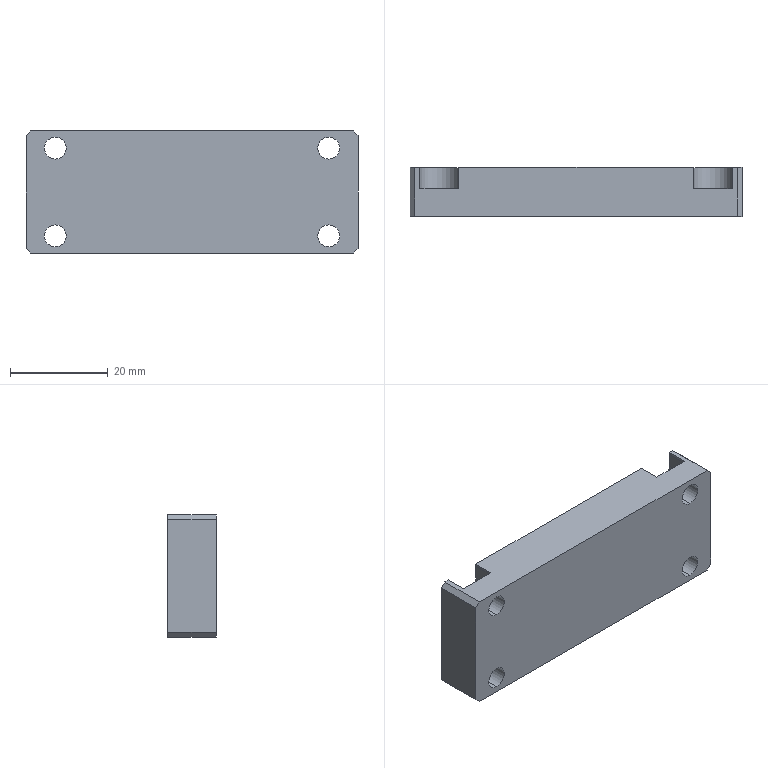Part | SolidWorks | features Chamfer 1, Extrusion 1, HoleWzd 1, ICE 1 | 1 solid | 44 faces | box 68 x 10 x 25 mm | volume 15689 mm3 | cylinder 22 | plane 22 | commonest cylinder face diameters 8 x14 4.5 x8
STEP:
#1=CARTESIAN_POINT('',(-28.,-5.,-11.25));
#2=VERTEX_POINT('',#1);
#3=CARTESIAN_POINT('',(-28.,-5.,-6.75));
#4=VERTEX_POINT('',#3);
#5=CARTESIAN_POINT('',(-28.,-5.,-9.));
#6=DIRECTION('',(0.,1.,0.));
#7=DIRECTION('',(0.,0.,1.));
#8=AXIS2_PLACEMENT_3D('',#5,#6,#7);
#9=CIRCLE('',#8,2.25);
#10=EDGE_CURVE('',#2,#4,#9,.T.);
#11=ORIENTED_EDGE('',*,*,#10,.F.);
#12=CARTESIAN_POINT('',(-28.,0.6,-11.25));
#13=VERTEX_POINT('',#12);
#14=CARTESIAN_POINT('',(-28.,5.,-11.25));
#15=DIRECTION('',(0.,1.,0.));
#16=VECTOR('',#15,1000.);
#17=LINE('',#14,#16);
#18=EDGE_CURVE('',#2,#13,#17,.T.);
#19=ORIENTED_EDGE('',*,*,#18,.T.);
#20=CARTESIAN_POINT('',(-28.,0.6,-6.75));
#21=VERTEX_POINT('',#20);
#22=CARTESIAN_POINT('',(-28.,0.6,-9.));
#23=DIRECTION('',(0.,1.,0.));
#24=DIRECTION('',(0.,0.,1.));
#25=AXIS2_PLACEMENT_3D('',#22,#23,#24);
#26=CIRCLE('',#25,2.25);
#27=EDGE_CURVE('',#13,#21,#26,.T.);
#28=ORIENTED_EDGE('',*,*,#27,.T.);
#29=CARTESIAN_POINT('',(-28.,5.,-6.75));
#30=DIRECTION('',(0.,1.,0.));
#31=VECTOR('',#30,1000.);
#32=LINE('',#29,#31);
#33=EDGE_CURVE('',#4,#21,#32,.T.);
#34=ORIENTED_EDGE('',*,*,#33,.F.);
#35=EDGE_LOOP('',(#11,#19,#28,#34));
#36=FACE_OUTER_BOUND('',#35,.T.);
#37=CARTESIAN_POINT('',(-28.,5.,-9.));
#38=DIRECTION('',(0.,1.,0.));
#39=DIRECTION('',(0.,0.,1.));
#40=AXIS2_PLACEMENT_3D('',#37,#38,#39);
#41=CYLINDRICAL_SURFACE('',#40,2.25);
#42=ADVANCED_FACE('',(#36),#41,.F.);
#43=CARTESIAN_POINT('',(-28.,-5.,6.75));
#44=VERTEX_POINT('',#43);
#45=CARTESIAN_POINT('',(-28.,-5.,11.25));
#46=VERTEX_POINT('',#45);
#47=CARTESIAN_POINT('',(-28.,-5.,9.));
#48=DIRECTION('',(0.,1.,0.));
#49=DIRECTION('',(0.,0.,1.));
#50=AXIS2_PLACEMENT_3D('',#47,#48,#49);
#51=CIRCLE('',#50,2.25);
#52=EDGE_CURVE('',#44,#46,#51,.T.);
#53=ORIENTED_EDGE('',*,*,#52,.F.);
#54=CARTESIAN_POINT('',(-28.,0.6,6.75));
#55=VERTEX_POINT('',#54);
#56=CARTESIAN_POINT('',(-28.,5.,6.75));
#57=DIRECTION('',(0.,1.,0.));
#58=VECTOR('',#57,1000.);
#59=LINE('',#56,#58);
#60=EDGE_CURVE('',#44,#55,#59,.T.);
#61=ORIENTED_EDGE('',*,*,#60,.T.);
#62=CARTESIAN_POINT('',(-28.,0.6,11.25));
#63=VERTEX_POINT('',#62);
#64=CARTESIAN_POINT('',(-28.,0.6,9.));
#65=DIRECTION('',(0.,1.,0.));
#66=DIRECTION('',(0.,0.,1.));
#67=AXIS2_PLACEMENT_3D('',#64,#65,#66);
#68=CIRCLE('',#67,2.25);
#69=EDGE_CURVE('',#55,#63,#68,.T.);
#70=ORIENTED_EDGE('',*,*,#69,.T.);
#71=CARTESIAN_POINT('',(-28.,5.,11.25));
#72=DIRECTION('',(0.,1.,0.));
#73=VECTOR('',#72,1000.);
#74=LINE('',#71,#73);
#75=EDGE_CURVE('',#46,#63,#74,.T.);
#76=ORIENTED_EDGE('',*,*,#75,.F.);
#77=EDGE_LOOP('',(#53,#61,#70,#76));
#78=FACE_OUTER_BOUND('',#77,.T.);
#79=CARTESIAN_POINT('',(-28.,5.,9.));
#80=DIRECTION('',(0.,1.,0.));
#81=DIRECTION('',(0.,0.,1.));
#82=AXIS2_PLACEMENT_3D('',#79,#80,#81);
#83=CYLINDRICAL_SURFACE('',#82,2.25);
#84=ADVANCED_FACE('',(#78),#83,.F.);
#85=CARTESIAN_POINT('',(28.,-5.,-11.25));
#86=VERTEX_POINT('',#85);
#87=CARTESIAN_POINT('',(28.,-5.,-6.75));
#88=VERTEX_POINT('',#87);
#89=CARTESIAN_POINT('',(28.,-5.,-9.));
#90=DIRECTION('',(0.,1.,0.));
#91=DIRECTION('',(0.,0.,1.));
#92=AXIS2_PLACEMENT_3D('',#89,#90,#91);
#93=CIRCLE('',#92,2.25);
#94=EDGE_CURVE('',#86,#88,#93,.T.);
#95=ORIENTED_EDGE('',*,*,#94,.F.);
#96=CARTESIAN_POINT('',(28.,0.6,-11.25));
#97=VERTEX_POINT('',#96);
#98=CARTESIAN_POINT('',(28.,5.,-11.25));
#99=DIRECTION('',(0.,1.,0.));
#100=VECTOR('',#99,1000.);
#101=LINE('',#98,#100);
#102=EDGE_CURVE('',#86,#97,#101,.T.);
#103=ORIENTED_EDGE('',*,*,#102,.T.);
#104=CARTESIAN_POINT('',(28.,0.6,-6.75));
#105=VERTEX_POINT('',#104);
#106=CARTESIAN_POINT('',(28.,0.6,-9.));
#107=DIRECTION('',(0.,1.,0.));
#108=DIRECTION('',(0.,0.,1.));
#109=AXIS2_PLACEMENT_3D('',#106,#107,#108);
#110=CIRCLE('',#109,2.25);
#111=EDGE_CURVE('',#97,#105,#110,.T.);
#112=ORIENTED_EDGE('',*,*,#111,.T.);
#113=CARTESIAN_POINT('',(28.,5.,-6.75));
#114=DIRECTION('',(0.,1.,0.));
#115=VECTOR('',#114,1000.);
#116=LINE('',#113,#115);
#117=EDGE_CURVE('',#88,#105,#116,.T.);
#118=ORIENTED_EDGE('',*,*,#117,.F.);
#119=EDGE_LOOP('',(#95,#103,#112,#118));
#120=FACE_OUTER_BOUND('',#119,.T.);
#121=CARTESIAN_POINT('',(28.,5.,-9.));
#122=DIRECTION('',(0.,1.,0.));
#123=DIRECTION('',(0.,0.,1.));
#124=AXIS2_PLACEMENT_3D('',#121,#122,#123);
#125=CYLINDRICAL_SURFACE('',#124,2.25);
#126=ADVANCED_FACE('',(#120),#125,.F.);
#127=CARTESIAN_POINT('',(28.,-5.,6.75));
#128=VERTEX_POINT('',#127);
#129=CARTESIAN_POINT('',(28.,-5.,11.25));
#130=VERTEX_POINT('',#129);
#131=CARTESIAN_POINT('',(28.,-5.,9.));
#132=DIRECTION('',(0.,1.,0.));
#133=DIRECTION('',(0.,0.,1.));
#134=AXIS2_PLACEMENT_3D('',#131,#132,#133);
#135=CIRCLE('',#134,2.25);
#136=EDGE_CURVE('',#128,#130,#135,.T.);
#137=ORIENTED_EDGE('',*,*,#136,.F.);
#138=CARTESIAN_POINT('',(28.,0.6,6.75));
#139=VERTEX_POINT('',#138);
#140=CARTESIAN_POINT('',(28.,5.,6.75));
#141=DIRECTION('',(0.,1.,0.));
#142=VECTOR('',#141,1000.);
#143=LINE('',#140,#142);
#144=EDGE_CURVE('',#128,#139,#143,.T.);
#145=ORIENTED_EDGE('',*,*,#144,.T.);
#146=CARTESIAN_POINT('',(28.,0.6,11.25));
#147=VERTEX_POINT('',#146);
#148=CARTESIAN_POINT('',(28.,0.6,9.));
#149=DIRECTION('',(0.,1.,0.));
#150=DIRECTION('',(0.,0.,1.));
#151=AXIS2_PLACEMENT_3D('',#148,#149,#150);
#152=CIRCLE('',#151,2.25);
#153=EDGE_CURVE('',#139,#147,#152,.T.);
#154=ORIENTED_EDGE('',*,*,#153,.T.);
#155=CARTESIAN_POINT('',(28.,5.,11.25));
#156=DIRECTION('',(0.,1.,0.));
#157=VECTOR('',#156,1000.);
#158=LINE('',#155,#157);
#159=EDGE_CURVE('',#130,#147,#158,.T.);
#160=ORIENTED_EDGE('',*,*,#159,.F.);
#161=EDGE_LOOP('',(#137,#145,#154,#160));
#162=FACE_OUTER_BOUND('',#161,.T.);
#163=CARTESIAN_POINT('',(28.,5.,9.));
#164=DIRECTION('',(0.,1.,0.));
#165=DIRECTION('',(0.,0.,1.));
#166=AXIS2_PLACEMENT_3D('',#163,#164,#165);
#167=CYLINDRICAL_SURFACE('',#166,2.25);
#168=ADVANCED_FACE('',(#162),#167,.F.);
#169=CARTESIAN_POINT('',(-28.,0.6,-5.));
#170=VERTEX_POINT('',#169);
#171=CARTESIAN_POINT('',(-24.,0.6,-9.));
#172=VERTEX_POINT('',#171);
#173=CARTESIAN_POINT('',(-28.,0.6,-9.));
#174=DIRECTION('',(0.,1.,0.));
#175=DIRECTION('',(0.,0.,1.));
#176=AXIS2_PLACEMENT_3D('',#173,#174,#175);
#177=CIRCLE('',#176,4.);
#178=EDGE_CURVE('',#170,#172,#177,.T.);
#179=ORIENTED_EDGE('',*,*,#178,.F.);
#180=CARTESIAN_POINT('',(-28.,5.,-5.));
#181=VERTEX_POINT('',#180);
#182=CARTESIAN_POINT('',(-28.,5.,-5.));
#183=DIRECTION('',(0.,1.,0.));
#184=VECTOR('',#183,1000.);
#185=LINE('',#182,#184);
#186=EDGE_CURVE('',#170,#181,#185,.T.);
#187=ORIENTED_EDGE('',*,*,#186,.T.);
#188=CARTESIAN_POINT('',(-24.,5.,-9.));
#189=VERTEX_POINT('',#188);
#190=CARTESIAN_POINT('',(-28.,5.,-9.));
#191=DIRECTION('',(0.,1.,0.));
#192=DIRECTION('',(0.,0.,1.));
#193=AXIS2_PLACEMENT_3D('',#190,#191,#192);
#194=CIRCLE('',#193,4.);
#195=EDGE_CURVE('',#181,#189,#194,.T.);
#196=ORIENTED_EDGE('',*,*,#195,.T.);
#197=CARTESIAN_POINT('',(-24.,-13.001,-9.));
#198=DIRECTION('',(0.,1.,0.));
#199=VECTOR('',#198,1000.);
#200=LINE('',#197,#199);
#201=EDGE_CURVE('',#172,#189,#200,.T.);
#202=ORIENTED_EDGE('',*,*,#201,.F.);
#203=EDGE_LOOP('',(#179,#187,#196,#202));
#204=FACE_OUTER_BOUND('',#203,.T.);
#205=CARTESIAN_POINT('',(-28.,5.,-9.));
#206=DIRECTION('',(0.,1.,0.));
#207=DIRECTION('',(0.,0.,1.));
#208=AXIS2_PLACEMENT_3D('',#205,#206,#207);
#209=CYLINDRICAL_SURFACE('',#208,4.);
#210=ADVANCED_FACE('',(#204),#209,.F.);
#211=CARTESIAN_POINT('',(28.,0.6,-5.));
#212=VERTEX_POINT('',#211);
#213=CARTESIAN_POINT('',(32.,0.6,-9.));
#214=VERTEX_POINT('',#213);
#215=CARTESIAN_POINT('',(28.,0.6,-9.));
#216=DIRECTION('',(0.,1.,0.));
#217=DIRECTION('',(0.,0.,1.));
#218=AXIS2_PLACEMENT_3D('',#215,#216,#217);
#219=CIRCLE('',#218,4.);
#220=EDGE_CURVE('',#212,#214,#219,.T.);
#221=ORIENTED_EDGE('',*,*,#220,.F.);
#222=CARTESIAN_POINT('',(28.,5.,-5.));
#223=VERTEX_POINT('',#222);
#224=CARTESIAN_POINT('',(28.,5.,-5.));
#225=DIRECTION('',(0.,1.,0.));
#226=VECTOR('',#225,1000.);
#227=LINE('',#224,#226);
#228=EDGE_CURVE('',#212,#223,#227,.T.);
#229=ORIENTED_EDGE('',*,*,#228,.T.);
#230=CARTESIAN_POINT('',(32.,5.,-9.));
#231=VERTEX_POINT('',#230);
#232=CARTESIAN_POINT('',(28.,5.,-9.));
#233=DIRECTION('',(0.,1.,0.));
#234=DIRECTION('',(0.,0.,1.));
#235=AXIS2_PLACEMENT_3D('',#232,#233,#234);
#236=CIRCLE('',#235,4.);
#237=EDGE_CURVE('',#223,#231,#236,.T.);
#238=ORIENTED_EDGE('',*,*,#237,.T.);
#239=CARTESIAN_POINT('',(32.,-13.001,-9.));
#240=DIRECTION('',(0.,1.,0.));
#241=VECTOR('',#240,1000.);
#242=LINE('',#239,#241);
#243=EDGE_CURVE('',#214,#231,#242,.T.);
#244=ORIENTED_EDGE('',*,*,#243,.F.);
#245=EDGE_LOOP('',(#221,#229,#238,#244));
#246=FACE_OUTER_BOUND('',#245,.T.);
#247=CARTESIAN_POINT('',(28.,5.,-9.));
#248=DIRECTION('',(0.,1.,0.));
#249=DIRECTION('',(0.,0.,1.));
#250=AXIS2_PLACEMENT_3D('',#247,#248,#249);
#251=CYLINDRICAL_SURFACE('',#250,4.);
#252=ADVANCED_FACE('',(#246),#251,.F.);
#253=CARTESIAN_POINT('',(32.,5.,9.));
#254=VERTEX_POINT('',#253);
#255=CARTESIAN_POINT('',(24.,5.,9.));
#256=VERTEX_POINT('',#255);
#257=CARTESIAN_POINT('',(28.,5.,9.));
#258=DIRECTION('',(0.,1.,0.));
#259=DIRECTION('',(0.,0.,1.));
#260=AXIS2_PLACEMENT_3D('',#257,#258,#259);
#261=CIRCLE('',#260,4.);
#262=EDGE_CURVE('',#254,#256,#261,.T.);
#263=ORIENTED_EDGE('',*,*,#262,.T.);
#264=CARTESIAN_POINT('',(24.,0.6,9.));
#265=VERTEX_POINT('',#264);
#266=CARTESIAN_POINT('',(24.,-13.001,9.));
#267=DIRECTION('',(0.,1.,0.));
#268=VECTOR('',#267,1000.);
#269=LINE('',#266,#268);
#270=EDGE_CURVE('',#265,#256,#269,.T.);
#271=ORIENTED_EDGE('',*,*,#270,.F.);
#272=CARTESIAN_POINT('',(32.,0.6,9.));
#273=VERTEX_POINT('',#272);
#274=CARTESIAN_POINT('',(28.,0.6,9.));
#275=DIRECTION('',(0.,1.,0.));
#276=DIRECTION('',(0.,0.,1.));
#277=AXIS2_PLACEMENT_3D('',#274,#275,#276);
#278=CIRCLE('',#277,4.);
#279=EDGE_CURVE('',#273,#265,#278,.T.);
#280=ORIENTED_EDGE('',*,*,#279,.F.);
#281=CARTESIAN_POINT('',(32.,-13.001,9.));
#282=DIRECTION('',(0.,1.,0.));
#283=VECTOR('',#282,1000.);
#284=LINE('',#281,#283);
#285=EDGE_CURVE('',#273,#254,#284,.T.);
#286=ORIENTED_EDGE('',*,*,#285,.T.);
#287=EDGE_LOOP('',(#263,#271,#280,#286));
#288=FACE_OUTER_BOUND('',#287,.T.);
#289=CARTESIAN_POINT('',(28.,5.,9.));
#290=DIRECTION('',(0.,1.,0.));
#291=DIRECTION('',(0.,0.,1.));
#292=AXIS2_PLACEMENT_3D('',#289,#290,#291);
#293=CYLINDRICAL_SURFACE('',#292,4.);
#294=ADVANCED_FACE('',(#288),#293,.F.);
#295=ORIENTED_EDGE('',*,*,#228,.F.);
#296=CARTESIAN_POINT('',(24.,0.6,-9.));
#297=VERTEX_POINT('',#296);
#298=CARTESIAN_POINT('',(28.,0.6,-9.));
#299=DIRECTION('',(0.,1.,0.));
#300=DIRECTION('',(0.,0.,1.));
#301=AXIS2_PLACEMENT_3D('',#298,#299,#300);
#302=CIRCLE('',#301,4.);
#303=EDGE_CURVE('',#297,#212,#302,.T.);
#304=ORIENTED_EDGE('',*,*,#303,.F.);
#305=CARTESIAN_POINT('',(24.,5.,-9.));
#306=VERTEX_POINT('',#305);
#307=CARTESIAN_POINT('',(24.,-13.001,-9.));
#308=DIRECTION('',(0.,1.,0.));
#309=VECTOR('',#308,1000.);
#310=LINE('',#307,#309);
#311=EDGE_CURVE('',#297,#306,#310,.T.);
#312=ORIENTED_EDGE('',*,*,#311,.T.);
#313=CARTESIAN_POINT('',(28.,5.,-9.));
#314=DIRECTION('',(0.,1.,0.));
#315=DIRECTION('',(0.,0.,1.));
#316=AXIS2_PLACEMENT_3D('',#313,#314,#315);
#317=CIRCLE('',#316,4.);
#318=EDGE_CURVE('',#306,#223,#317,.T.);
#319=ORIENTED_EDGE('',*,*,#318,.T.);
#320=EDGE_LOOP('',(#295,#304,#312,#319));
#321=FACE_OUTER_BOUND('',#320,.T.);
#322=CARTESIAN_POINT('',(28.,5.,-9.));
#323=DIRECTION('',(0.,1.,0.));
#324=DIRECTION('',(0.,0.,1.));
#325=AXIS2_PLACEMENT_3D('',#322,#323,#324);
#326=CYLINDRICAL_SURFACE('',#325,4.);
#327=ADVANCED_FACE('',(#321),#326,.F.);
#328=CARTESIAN_POINT('',(-24.,5.,9.));
#329=VERTEX_POINT('',#328);
#330=CARTESIAN_POINT('',(-32.,5.,9.));
#331=VERTEX_POINT('',#330);
#332=CARTESIAN_POINT('',(-28.,5.,9.));
#333=DIRECTION('',(0.,1.,0.));
#334=DIRECTION('',(0.,0.,1.));
#335=AXIS2_PLACEMENT_3D('',#332,#333,#334);
#336=CIRCLE('',#335,4.);
#337=EDGE_CURVE('',#329,#331,#336,.T.);
#338=ORIENTED_EDGE('',*,*,#337,.T.);
#339=CARTESIAN_POINT('',(-32.,0.6,9.));
#340=VERTEX_POINT('',#339);
#341=CARTESIAN_POINT('',(-32.,-13.001,9.));
#342=DIRECTION('',(0.,1.,0.));
#343=VECTOR('',#342,1000.);
#344=LINE('',#341,#343);
#345=EDGE_CURVE('',#340,#331,#344,.T.);
#346=ORIENTED_EDGE('',*,*,#345,.F.);
#347=CARTESIAN_POINT('',(-24.,0.6,9.));
#348=VERTEX_POINT('',#347);
#349=CARTESIAN_POINT('',(-28.,0.6,9.));
#350=DIRECTION('',(0.,1.,0.));
#351=DIRECTION('',(0.,0.,1.));
#352=AXIS2_PLACEMENT_3D('',#349,#350,#351);
#353=CIRCLE('',#352,4.);
#354=EDGE_CURVE('',#348,#340,#353,.T.);
#355=ORIENTED_EDGE('',*,*,#354,.F.);
#356=CARTESIAN_POINT('',(-24.,-13.001,9.));
#357=DIRECTION('',(0.,1.,0.));
#358=VECTOR('',#357,1000.);
#359=LINE('',#356,#358);
#360=EDGE_CURVE('',#348,#329,#359,.T.);
#361=ORIENTED_EDGE('',*,*,#360,.T.);
#362=EDGE_LOOP('',(#338,#346,#355,#361));
#363=FACE_OUTER_BOUND('',#362,.T.);
#364=CARTESIAN_POINT('',(-28.,5.,9.));
#365=DIRECTION('',(0.,1.,0.));
#366=DIRECTION('',(0.,0.,1.));
#367=AXIS2_PLACEMENT_3D('',#364,#365,#366);
#368=CYLINDRICAL_SURFACE('',#367,4.);
#369=ADVANCED_FACE('',(#363),#368,.F.);
#370=ORIENTED_EDGE('',*,*,#186,.F.);
#371=CARTESIAN_POINT('',(-32.,0.6,-9.));
#372=VERTEX_POINT('',#371);
#373=CARTESIAN_POINT('',(-28.,0.6,-9.));
#374=DIRECTION('',(0.,1.,0.));
#375=DIRECTION('',(0.,0.,1.));
#376=AXIS2_PLACEMENT_3D('',#373,#374,#375);
#377=CIRCLE('',#376,4.);
#378=EDGE_CURVE('',#372,#170,#377,.T.);
#379=ORIENTED_EDGE('',*,*,#378,.F.);
#380=CARTESIAN_POINT('',(-32.,5.,-9.));
#381=VERTEX_POINT('',#380);
#382=CARTESIAN_POINT('',(-32.,-13.001,-9.));
#383=DIRECTION('',(0.,1.,0.));
#384=VECTOR('',#383,1000.);
#385=LINE('',#382,#384);
#386=EDGE_CURVE('',#372,#381,#385,.T.);
#387=ORIENTED_EDGE('',*,*,#386,.T.);
#388=CARTESIAN_POINT('',(-28.,5.,-9.));
#389=DIRECTION('',(0.,1.,0.));
#390=DIRECTION('',(0.,0.,1.));
#391=AXIS2_PLACEMENT_3D('',#388,#389,#390);
#392=CIRCLE('',#391,4.);
#393=EDGE_CURVE('',#381,#181,#392,.T.);
#394=ORIENTED_EDGE('',*,*,#393,.T.);
#395=EDGE_LOOP('',(#370,#379,#387,#394));
#396=FACE_OUTER_BOUND('',#395,.T.);
#397=CARTESIAN_POINT('',(-28.,5.,-9.));
#398=DIRECTION('',(0.,1.,0.));
#399=DIRECTION('',(0.,0.,1.));
#400=AXIS2_PLACEMENT_3D('',#397,#398,#399);
#401=CYLINDRICAL_SURFACE('',#400,4.);
#402=ADVANCED_FACE('',(#396),#401,.F.);
#403=CARTESIAN_POINT('',(34.,-5.,11.5));
#404=VERTEX_POINT('',#403);
#405=CARTESIAN_POINT('',(34.,-5.,-11.5));
#406=VERTEX_POINT('',#405);
#407=CARTESIAN_POINT('',(34.,-5.,-12.5));
#408=DIRECTION('',(0.,0.,-1.));
#409=VECTOR('',#408,1000.);
#410=LINE('',#407,#409);
#411=EDGE_CURVE('',#404,#406,#410,.T.);
#412=ORIENTED_EDGE('',*,*,#411,.T.);
#413=CARTESIAN_POINT('',(34.,5.,-11.5));
#414=VERTEX_POINT('',#413);
#415=CARTESIAN_POINT('',(34.,5.,-11.5));
#416=DIRECTION('',(0.,1.,0.));
#417=VECTOR('',#416,1000.);
#418=LINE('',#415,#417);
#419=EDGE_CURVE('',#406,#414,#418,.T.);
#420=ORIENTED_EDGE('',*,*,#419,.T.);
#421=CARTESIAN_POINT('',(34.,5.,11.5));
#422=VERTEX_POINT('',#421);
#423=CARTESIAN_POINT('',(34.,5.,-12.5));
#424=DIRECTION('',(0.,0.,-1.));
#425=VECTOR('',#424,1000.);
#426=LINE('',#423,#425);
#427=EDGE_CURVE('',#422,#414,#426,.T.);
#428=ORIENTED_EDGE('',*,*,#427,.F.);
#429=CARTESIAN_POINT('',(34.,5.,11.5));
#430=DIRECTION('',(0.,-1.,0.));
#431=VECTOR('',#430,1000.);
#432=LINE('',#429,#431);
#433=EDGE_CURVE('',#422,#404,#432,.T.);
#434=ORIENTED_EDGE('',*,*,#433,.T.);
#435=EDGE_LOOP('',(#412,#420,#428,#434));
#436=FACE_OUTER_BOUND('',#435,.T.);
#437=CARTESIAN_POINT('',(34.,5.,-12.5));
#438=DIRECTION('',(-1.,0.,0.));
#439=DIRECTION('',(0.,0.,1.));
#440=AXIS2_PLACEMENT_3D('',#437,#438,#439);
#441=PLANE('',#440);
#442=ADVANCED_FACE('',(#436),#441,.F.);
#443=CARTESIAN_POINT('',(33.,5.,-12.5));
#444=VERTEX_POINT('',#443);
#445=CARTESIAN_POINT('',(31.969,5.,-12.5));
#446=VERTEX_POINT('',#445);
#447=CARTESIAN_POINT('',(-34.,5.,-12.5));
#448=DIRECTION('',(-1.,0.,0.));
#449=VECTOR('',#448,1000.);
#450=LINE('',#447,#449);
#451=EDGE_CURVE('',#444,#446,#450,.T.);
#452=ORIENTED_EDGE('',*,*,#451,.F.);
#453=CARTESIAN_POINT('',(33.,-5.,-12.5));
#454=VERTEX_POINT('',#453);
#455=CARTESIAN_POINT('',(33.,5.,-12.5));
#456=DIRECTION('',(0.,-1.,0.));
#457=VECTOR('',#456,1000.);
#458=LINE('',#455,#457);
#459=EDGE_CURVE('',#444,#454,#458,.T.);
#460=ORIENTED_EDGE('',*,*,#459,.T.);
#461=CARTESIAN_POINT('',(-33.,-5.,-12.5));
#462=VERTEX_POINT('',#461);
#463=CARTESIAN_POINT('',(-34.,-5.,-12.5));
#464=DIRECTION('',(-1.,0.,0.));
#465=VECTOR('',#464,1000.);
#466=LINE('',#463,#465);
#467=EDGE_CURVE('',#454,#462,#466,.T.);
#468=ORIENTED_EDGE('',*,*,#467,.T.);
#469=CARTESIAN_POINT('',(-33.,5.,-12.5));
#470=VERTEX_POINT('',#469);
#471=CARTESIAN_POINT('',(-33.,5.,-12.5));
#472=DIRECTION('',(0.,1.,0.));
#473=VECTOR('',#472,1000.);
#474=LINE('',#471,#473);
#475=EDGE_CURVE('',#462,#470,#474,.T.);
#476=ORIENTED_EDGE('',*,*,#475,.T.);
#477=CARTESIAN_POINT('',(-31.969,5.,-12.5));
#478=VERTEX_POINT('',#477);
#479=CARTESIAN_POINT('',(-34.,5.,-12.5));
#480=DIRECTION('',(-1.,0.,0.));
#481=VECTOR('',#480,1000.);
#482=LINE('',#479,#481);
#483=EDGE_CURVE('',#478,#470,#482,.T.);
#484=ORIENTED_EDGE('',*,*,#483,.F.);
#485=CARTESIAN_POINT('',(-31.969,0.6,-12.5));
#486=VERTEX_POINT('',#485);
#487=CARTESIAN_POINT('',(-31.969,-13.001,-12.5));
#488=DIRECTION('',(0.,-1.,0.));
#489=VECTOR('',#488,1000.);
#490=LINE('',#487,#489);
#491=EDGE_CURVE('',#478,#486,#490,.T.);
#492=ORIENTED_EDGE('',*,*,#491,.T.);
#493=CARTESIAN_POINT('',(-24.031,0.6,-12.5));
#494=VERTEX_POINT('',#493);
#495=CARTESIAN_POINT('',(-34.,0.6,-12.5));
#496=DIRECTION('',(1.,0.,0.));
#497=VECTOR('',#496,1000.);
#498=LINE('',#495,#497);
#499=EDGE_CURVE('',#486,#494,#498,.T.);
#500=ORIENTED_EDGE('',*,*,#499,.T.);
#501=CARTESIAN_POINT('',(-24.031,5.,-12.5));
#502=VERTEX_POINT('',#501);
#503=CARTESIAN_POINT('',(-24.031,-13.001,-12.5));
#504=DIRECTION('',(0.,1.,0.));
#505=VECTOR('',#504,1000.);
#506=LINE('',#503,#505);
#507=EDGE_CURVE('',#494,#502,#506,.T.);
#508=ORIENTED_EDGE('',*,*,#507,.T.);
#509=CARTESIAN_POINT('',(24.031,5.,-12.5));
#510=VERTEX_POINT('',#509);
#511=CARTESIAN_POINT('',(-34.,5.,-12.5));
#512=DIRECTION('',(-1.,0.,0.));
#513=VECTOR('',#512,1000.);
#514=LINE('',#511,#513);
#515=EDGE_CURVE('',#510,#502,#514,.T.);
#516=ORIENTED_EDGE('',*,*,#515,.F.);
#517=CARTESIAN_POINT('',(24.031,0.6,-12.5));
#518=VERTEX_POINT('',#517);
#519=CARTESIAN_POINT('',(24.031,-13.001,-12.5));
#520=DIRECTION('',(0.,-1.,0.));
#521=VECTOR('',#520,1000.);
#522=LINE('',#519,#521);
#523=EDGE_CURVE('',#510,#518,#522,.T.);
#524=ORIENTED_EDGE('',*,*,#523,.T.);
#525=CARTESIAN_POINT('',(31.969,0.6,-12.5));
#526=VERTEX_POINT('',#525);
#527=CARTESIAN_POINT('',(-34.,0.6,-12.5));
#528=DIRECTION('',(1.,0.,0.));
#529=VECTOR('',#528,1000.);
#530=LINE('',#527,#529);
#531=EDGE_CURVE('',#518,#526,#530,.T.);
#532=ORIENTED_EDGE('',*,*,#531,.T.);
#533=CARTESIAN_POINT('',(31.969,-13.001,-12.5));
#534=DIRECTION('',(0.,1.,0.));
#535=VECTOR('',#534,1000.);
#536=LINE('',#533,#535);
#537=EDGE_CURVE('',#526,#446,#536,.T.);
#538=ORIENTED_EDGE('',*,*,#537,.T.);
#539=EDGE_LOOP('',(#452,#460,#468,#476,#484,#492,#500,#508,#516,#524,#532,#538));
#540=FACE_OUTER_BOUND('',#539,.T.);
#541=CARTESIAN_POINT('',(-34.,5.,-12.5));
#542=DIRECTION('',(0.,0.,1.));
#543=DIRECTION('',(1.,0.,0.));
#544=AXIS2_PLACEMENT_3D('',#541,#542,#543);
#545=PLANE('',#544);
#546=ADVANCED_FACE('',(#540),#545,.F.);
#547=CARTESIAN_POINT('',(-34.,-5.,-11.5));
#548=VERTEX_POINT('',#547);
#549=CARTESIAN_POINT('',(-34.,-5.,11.5));
#550=VERTEX_POINT('',#549);
#551=CARTESIAN_POINT('',(-34.,-5.,-12.5));
#552=DIRECTION('',(0.,0.,1.));
#553=VECTOR('',#552,1000.);
#554=LINE('',#551,#553);
#555=EDGE_CURVE('',#548,#550,#554,.T.);
#556=ORIENTED_EDGE('',*,*,#555,.T.);
#557=CARTESIAN_POINT('',(-34.,5.,11.5));
#558=VERTEX_POINT('',#557);
#559=CARTESIAN_POINT('',(-34.,5.,11.5));
#560=DIRECTION('',(0.,1.,0.));
#561=VECTOR('',#560,1000.);
#562=LINE('',#559,#561);
#563=EDGE_CURVE('',#550,#558,#562,.T.);
#564=ORIENTED_EDGE('',*,*,#563,.T.);
#565=CARTESIAN_POINT('',(-34.,5.,-11.5));
#566=VERTEX_POINT('',#565);
#567=CARTESIAN_POINT('',(-34.,5.,-12.5));
#568=DIRECTION('',(0.,0.,1.));
#569=VECTOR('',#568,1000.);
#570=LINE('',#567,#569);
#571=EDGE_CURVE('',#566,#558,#570,.T.);
#572=ORIENTED_EDGE('',*,*,#571,.F.);
#573=CARTESIAN_POINT('',(-34.,5.,-11.5));
#574=DIRECTION('',(0.,-1.,0.));
#575=VECTOR('',#574,1000.);
#576=LINE('',#573,#575);
#577=EDGE_CURVE('',#566,#548,#576,.T.);
#578=ORIENTED_EDGE('',*,*,#577,.T.);
#579=EDGE_LOOP('',(#556,#564,#572,#578));
#580=FACE_OUTER_BOUND('',#579,.T.);
#581=CARTESIAN_POINT('',(-34.,5.,-12.5));
#582=DIRECTION('',(1.,0.,0.));
#583=DIRECTION('',(0.,0.,-1.));
#584=AXIS2_PLACEMENT_3D('',#581,#582,#583);
#585=PLANE('',#584);
#586=ADVANCED_FACE('',(#580),#585,.F.);
#587=CARTESIAN_POINT('',(-33.,-5.,12.5));
#588=VERTEX_POINT('',#587);
#589=CARTESIAN_POINT('',(33.,-5.,12.5));
#590=VERTEX_POINT('',#589);
#591=CARTESIAN_POINT('',(-34.,-5.,12.5));
#592=DIRECTION('',(1.,0.,0.));
#593=VECTOR('',#592,1000.);
#594=LINE('',#591,#593);
#595=EDGE_CURVE('',#588,#590,#594,.T.);
#596=ORIENTED_EDGE('',*,*,#595,.T.);
#597=CARTESIAN_POINT('',(33.,5.,12.5));
#598=VERTEX_POINT('',#597);
#599=CARTESIAN_POINT('',(33.,5.,12.5));
#600=DIRECTION('',(0.,1.,0.));
#601=VECTOR('',#600,1000.);
#602=LINE('',#599,#601);
#603=EDGE_CURVE('',#590,#598,#602,.T.);
#604=ORIENTED_EDGE('',*,*,#603,.T.);
#605=CARTESIAN_POINT('',(31.969,5.,12.5));
#606=VERTEX_POINT('',#605);
#607=CARTESIAN_POINT('',(-34.,5.,12.5));
#608=DIRECTION('',(1.,0.,0.));
#609=VECTOR('',#608,1000.);
#610=LINE('',#607,#609);
#611=EDGE_CURVE('',#606,#598,#610,.T.);
#612=ORIENTED_EDGE('',*,*,#611,.F.);
#613=CARTESIAN_POINT('',(31.969,0.6,12.5));
#614=VERTEX_POINT('',#613);
#615=CARTESIAN_POINT('',(31.969,-13.001,12.5));
#616=DIRECTION('',(0.,-1.,0.));
#617=VECTOR('',#616,1000.);
#618=LINE('',#615,#617);
#619=EDGE_CURVE('',#606,#614,#618,.T.);
#620=ORIENTED_EDGE('',*,*,#619,.T.);
#621=CARTESIAN_POINT('',(24.031,0.6,12.5));
#622=VERTEX_POINT('',#621);
#623=CARTESIAN_POINT('',(-34.,0.6,12.5));
#624=DIRECTION('',(-1.,0.,0.));
#625=VECTOR('',#624,1000.);
#626=LINE('',#623,#625);
#627=EDGE_CURVE('',#614,#622,#626,.T.);
#628=ORIENTED_EDGE('',*,*,#627,.T.);
#629=CARTESIAN_POINT('',(24.031,5.,12.5));
#630=VERTEX_POINT('',#629);
#631=CARTESIAN_POINT('',(24.031,-13.001,12.5));
#632=DIRECTION('',(0.,1.,0.));
#633=VECTOR('',#632,1000.);
#634=LINE('',#631,#633);
#635=EDGE_CURVE('',#622,#630,#634,.T.);
#636=ORIENTED_EDGE('',*,*,#635,.T.);
#637=CARTESIAN_POINT('',(-24.031,5.,12.5));
#638=VERTEX_POINT('',#637);
#639=CARTESIAN_POINT('',(-34.,5.,12.5));
#640=DIRECTION('',(1.,0.,0.));
#641=VECTOR('',#640,1000.);
#642=LINE('',#639,#641);
#643=EDGE_CURVE('',#638,#630,#642,.T.);
#644=ORIENTED_EDGE('',*,*,#643,.F.);
#645=CARTESIAN_POINT('',(-24.031,0.6,12.5));
#646=VERTEX_POINT('',#645);
#647=CARTESIAN_POINT('',(-24.031,-13.001,12.5));
#648=DIRECTION('',(0.,-1.,0.));
#649=VECTOR('',#648,1000.);
#650=LINE('',#647,#649);
#651=EDGE_CURVE('',#638,#646,#650,.T.);
#652=ORIENTED_EDGE('',*,*,#651,.T.);
#653=CARTESIAN_POINT('',(-31.969,0.6,12.5));
#654=VERTEX_POINT('',#653);
#655=CARTESIAN_POINT('',(-34.,0.6,12.5));
#656=DIRECTION('',(-1.,0.,0.));
#657=VECTOR('',#656,1000.);
#658=LINE('',#655,#657);
#659=EDGE_CURVE('',#646,#654,#658,.T.);
#660=ORIENTED_EDGE('',*,*,#659,.T.);
#661=CARTESIAN_POINT('',(-31.969,5.,12.5));
#662=VERTEX_POINT('',#661);
#663=CARTESIAN_POINT('',(-31.969,-13.001,12.5));
#664=DIRECTION('',(0.,1.,0.));
#665=VECTOR('',#664,1000.);
#666=LINE('',#663,#665);
#667=EDGE_CURVE('',#654,#662,#666,.T.);
#668=ORIENTED_EDGE('',*,*,#667,.T.);
#669=CARTESIAN_POINT('',(-33.,5.,12.5));
#670=VERTEX_POINT('',#669);
#671=CARTESIAN_POINT('',(-34.,5.,12.5));
#672=DIRECTION('',(1.,0.,0.));
#673=VECTOR('',#672,1000.);
#674=LINE('',#671,#673);
#675=EDGE_CURVE('',#670,#662,#674,.T.);
#676=ORIENTED_EDGE('',*,*,#675,.F.);
#677=CARTESIAN_POINT('',(-33.,5.,12.5));
#678=DIRECTION('',(0.,-1.,0.));
#679=VECTOR('',#678,1000.);
#680=LINE('',#677,#679);
#681=EDGE_CURVE('',#670,#588,#680,.T.);
#682=ORIENTED_EDGE('',*,*,#681,.T.);
#683=EDGE_LOOP('',(#596,#604,#612,#620,#628,#636,#644,#652,#660,#668,#676,#682));
#684=FACE_OUTER_BOUND('',#683,.T.);
#685=CARTESIAN_POINT('',(-34.,5.,12.5));
#686=DIRECTION('',(0.,0.,-1.));
#687=DIRECTION('',(-1.,0.,0.));
#688=AXIS2_PLACEMENT_3D('',#685,#686,#687);
#689=PLANE('',#688);
#690=ADVANCED_FACE('',(#684),#689,.F.);
#691=ORIENTED_EDGE('',*,*,#427,.T.);
#692=CARTESIAN_POINT('',(22.75,5.,-22.75));
#693=DIRECTION('',(-0.7071,0.,-0.7071));
#694=VECTOR('',#693,1000.);
#695=LINE('',#692,#694);
#696=EDGE_CURVE('',#414,#444,#695,.T.);
#697=ORIENTED_EDGE('',*,*,#696,.T.);
#698=ORIENTED_EDGE('',*,*,#451,.T.);
#699=CARTESIAN_POINT('',(32.,5.,-12.));
#700=VERTEX_POINT('',#699);
#701=CARTESIAN_POINT('',(28.,5.,-12.));
#702=DIRECTION('',(0.,1.,0.));
#703=DIRECTION('',(0.,0.,-1.));
#704=AXIS2_PLACEMENT_3D('',#701,#702,#703);
#705=CIRCLE('',#704,4.);
#706=EDGE_CURVE('',#700,#446,#705,.T.);
#707=ORIENTED_EDGE('',*,*,#706,.F.);
#708=CARTESIAN_POINT('',(32.,5.,-9.));
#709=DIRECTION('',(0.,0.,-1.));
#710=VECTOR('',#709,1000.);
#711=LINE('',#708,#710);
#712=EDGE_CURVE('',#231,#700,#711,.T.);
#713=ORIENTED_EDGE('',*,*,#712,.F.);
#714=ORIENTED_EDGE('',*,*,#237,.F.);
#715=ORIENTED_EDGE('',*,*,#318,.F.);
#716=CARTESIAN_POINT('',(24.,5.,-12.));
#717=VERTEX_POINT('',#716);
#718=CARTESIAN_POINT('',(24.,5.,-9.));
#719=DIRECTION('',(0.,0.,1.));
#720=VECTOR('',#719,1000.);
#721=LINE('',#718,#720);
#722=EDGE_CURVE('',#717,#306,#721,.T.);
#723=ORIENTED_EDGE('',*,*,#722,.F.);
#724=CARTESIAN_POINT('',(28.,5.,-12.));
#725=DIRECTION('',(0.,1.,0.));
#726=DIRECTION('',(0.,0.,-1.));
#727=AXIS2_PLACEMENT_3D('',#724,#725,#726);
#728=CIRCLE('',#727,4.);
#729=EDGE_CURVE('',#510,#717,#728,.T.);
#730=ORIENTED_EDGE('',*,*,#729,.F.);
#731=ORIENTED_EDGE('',*,*,#515,.T.);
#732=CARTESIAN_POINT('',(-24.,5.,-12.));
#733=VERTEX_POINT('',#732);
#734=CARTESIAN_POINT('',(-28.,5.,-12.));
#735=DIRECTION('',(0.,1.,0.));
#736=DIRECTION('',(0.,0.,1.));
#737=AXIS2_PLACEMENT_3D('',#734,#735,#736);
#738=CIRCLE('',#737,4.);
#739=EDGE_CURVE('',#733,#502,#738,.T.);
#740=ORIENTED_EDGE('',*,*,#739,.F.);
#741=CARTESIAN_POINT('',(-24.,5.,-9.));
#742=DIRECTION('',(0.,0.,-1.));
#743=VECTOR('',#742,1000.);
#744=LINE('',#741,#743);
#745=EDGE_CURVE('',#189,#733,#744,.T.);
#746=ORIENTED_EDGE('',*,*,#745,.F.);
#747=ORIENTED_EDGE('',*,*,#195,.F.);
#748=ORIENTED_EDGE('',*,*,#393,.F.);
#749=CARTESIAN_POINT('',(-32.,5.,-12.));
#750=VERTEX_POINT('',#749);
#751=CARTESIAN_POINT('',(-32.,5.,-9.));
#752=DIRECTION('',(0.,0.,1.));
#753=VECTOR('',#752,1000.);
#754=LINE('',#751,#753);
#755=EDGE_CURVE('',#750,#381,#754,.T.);
#756=ORIENTED_EDGE('',*,*,#755,.F.);
#757=CARTESIAN_POINT('',(-28.,5.,-12.));
#758=DIRECTION('',(0.,1.,0.));
#759=DIRECTION('',(0.,0.,1.));
#760=AXIS2_PLACEMENT_3D('',#757,#758,#759);
#761=CIRCLE('',#760,4.);
#762=EDGE_CURVE('',#478,#750,#761,.T.);
#763=ORIENTED_EDGE('',*,*,#762,.F.);
#764=ORIENTED_EDGE('',*,*,#483,.T.);
#765=CARTESIAN_POINT('',(-22.75,5.,-22.75));
#766=DIRECTION('',(-0.7071,0.,0.7071));
#767=VECTOR('',#766,1000.);
#768=LINE('',#765,#767);
#769=EDGE_CURVE('',#470,#566,#768,.T.);
#770=ORIENTED_EDGE('',*,*,#769,.T.);
#771=ORIENTED_EDGE('',*,*,#571,.T.);
#772=CARTESIAN_POINT('',(-22.75,5.,22.75));
#773=DIRECTION('',(0.7071,0.,0.7071));
#774=VECTOR('',#773,1000.);
#775=LINE('',#772,#774);
#776=EDGE_CURVE('',#558,#670,#775,.T.);
#777=ORIENTED_EDGE('',*,*,#776,.T.);
#778=ORIENTED_EDGE('',*,*,#675,.T.);
#779=CARTESIAN_POINT('',(-32.,5.,12.));
#780=VERTEX_POINT('',#779);
#781=CARTESIAN_POINT('',(-28.,5.,12.));
#782=DIRECTION('',(0.,1.,0.));
#783=DIRECTION('',(0.,0.,-1.));
#784=AXIS2_PLACEMENT_3D('',#781,#782,#783);
#785=CIRCLE('',#784,4.);
#786=EDGE_CURVE('',#780,#662,#785,.T.);
#787=ORIENTED_EDGE('',*,*,#786,.F.);
#788=CARTESIAN_POINT('',(-32.,5.,9.));
#789=DIRECTION('',(0.,0.,1.));
#790=VECTOR('',#789,1000.);
#791=LINE('',#788,#790);
#792=EDGE_CURVE('',#331,#780,#791,.T.);
#793=ORIENTED_EDGE('',*,*,#792,.F.);
#794=ORIENTED_EDGE('',*,*,#337,.F.);
#795=CARTESIAN_POINT('',(-24.,5.,12.));
#796=VERTEX_POINT('',#795);
#797=CARTESIAN_POINT('',(-24.,5.,9.));
#798=DIRECTION('',(0.,0.,-1.));
#799=VECTOR('',#798,1000.);
#800=LINE('',#797,#799);
#801=EDGE_CURVE('',#796,#329,#800,.T.);
#802=ORIENTED_EDGE('',*,*,#801,.F.);
#803=CARTESIAN_POINT('',(-28.,5.,12.));
#804=DIRECTION('',(0.,1.,0.));
#805=DIRECTION('',(0.,0.,-1.));
#806=AXIS2_PLACEMENT_3D('',#803,#804,#805);
#807=CIRCLE('',#806,4.);
#808=EDGE_CURVE('',#638,#796,#807,.T.);
#809=ORIENTED_EDGE('',*,*,#808,.F.);
#810=ORIENTED_EDGE('',*,*,#643,.T.);
#811=CARTESIAN_POINT('',(24.,5.,12.));
#812=VERTEX_POINT('',#811);
#813=CARTESIAN_POINT('',(28.,5.,12.));
#814=DIRECTION('',(0.,1.,0.));
#815=DIRECTION('',(0.,0.,1.));
#816=AXIS2_PLACEMENT_3D('',#813,#814,#815);
#817=CIRCLE('',#816,4.);
#818=EDGE_CURVE('',#812,#630,#817,.T.);
#819=ORIENTED_EDGE('',*,*,#818,.F.);
#820=CARTESIAN_POINT('',(24.,5.,9.));
#821=DIRECTION('',(0.,0.,1.));
#822=VECTOR('',#821,1000.);
#823=LINE('',#820,#822);
#824=EDGE_CURVE('',#256,#812,#823,.T.);
#825=ORIENTED_EDGE('',*,*,#824,.F.);
#826=ORIENTED_EDGE('',*,*,#262,.F.);
#827=CARTESIAN_POINT('',(32.,5.,12.));
#828=VERTEX_POINT('',#827);
#829=CARTESIAN_POINT('',(32.,5.,9.));
#830=DIRECTION('',(0.,0.,-1.));
#831=VECTOR('',#830,1000.);
#832=LINE('',#829,#831);
#833=EDGE_CURVE('',#828,#254,#832,.T.);
#834=ORIENTED_EDGE('',*,*,#833,.F.);
#835=CARTESIAN_POINT('',(28.,5.,12.));
#836=DIRECTION('',(0.,1.,0.));
#837=DIRECTION('',(0.,0.,1.));
#838=AXIS2_PLACEMENT_3D('',#835,#836,#837);
#839=CIRCLE('',#838,4.);
#840=EDGE_CURVE('',#606,#828,#839,.T.);
#841=ORIENTED_EDGE('',*,*,#840,.F.);
#842=ORIENTED_EDGE('',*,*,#611,.T.);
#843=CARTESIAN_POINT('',(22.75,5.,22.75));
#844=DIRECTION('',(0.7071,0.,-0.7071));
#845=VECTOR('',#844,1000.);
#846=LINE('',#843,#845);
#847=EDGE_CURVE('',#598,#422,#846,.T.);
#848=ORIENTED_EDGE('',*,*,#847,.T.);
#849=EDGE_LOOP('',(#691,#697,#698,#707,#713,#714,#715,#723,#730,#731,#740,#746,#747,#748,#756,#763,#764,#770,#771,#777,#778,#787,#793,#794,#802,#809,#810,#819,#825,#826,#834,#841,#842,#848));
#850=FACE_OUTER_BOUND('',#849,.T.);
#851=CARTESIAN_POINT('',(0.,5.,0.));
#852=DIRECTION('',(0.,1.,0.));
#853=DIRECTION('',(0.,0.,1.));
#854=AXIS2_PLACEMENT_3D('',#851,#852,#853);
#855=PLANE('',#854);
#856=ADVANCED_FACE('',(#850),#855,.T.);
#857=CARTESIAN_POINT('',(-28.,-5.,-9.));
#858=DIRECTION('',(0.,1.,0.));
#859=DIRECTION('',(0.,0.,1.));
#860=AXIS2_PLACEMENT_3D('',#857,#858,#859);
#861=CIRCLE('',#860,2.25);
#862=EDGE_CURVE('',#4,#2,#861,.T.);
#863=ORIENTED_EDGE('',*,*,#862,.T.);
#864=ORIENTED_EDGE('',*,*,#10,.T.);
#865=EDGE_LOOP('',(#863,#864));
#866=FACE_BOUND('',#865,.T.);
#867=CARTESIAN_POINT('',(-28.,-5.,9.));
#868=DIRECTION('',(0.,1.,0.));
#869=DIRECTION('',(0.,0.,1.));
#870=AXIS2_PLACEMENT_3D('',#867,#868,#869);
#871=CIRCLE('',#870,2.25);
#872=EDGE_CURVE('',#46,#44,#871,.T.);
#873=ORIENTED_EDGE('',*,*,#872,.T.);
#874=ORIENTED_EDGE('',*,*,#52,.T.);
#875=EDGE_LOOP('',(#873,#874));
#876=FACE_BOUND('',#875,.T.);
#877=CARTESIAN_POINT('',(28.,-5.,-9.));
#878=DIRECTION('',(0.,1.,0.));
#879=DIRECTION('',(0.,0.,1.));
#880=AXIS2_PLACEMENT_3D('',#877,#878,#879);
#881=CIRCLE('',#880,2.25);
#882=EDGE_CURVE('',#88,#86,#881,.T.);
#883=ORIENTED_EDGE('',*,*,#882,.T.);
#884=ORIENTED_EDGE('',*,*,#94,.T.);
#885=EDGE_LOOP('',(#883,#884));
#886=FACE_BOUND('',#885,.T.);
#887=CARTESIAN_POINT('',(28.,-5.,9.));
#888=DIRECTION('',(0.,1.,0.));
#889=DIRECTION('',(0.,0.,1.));
#890=AXIS2_PLACEMENT_3D('',#887,#888,#889);
#891=CIRCLE('',#890,2.25);
#892=EDGE_CURVE('',#130,#128,#891,.T.);
#893=ORIENTED_EDGE('',*,*,#892,.T.);
#894=ORIENTED_EDGE('',*,*,#136,.T.);
#895=EDGE_LOOP('',(#893,#894));
#896=FACE_BOUND('',#895,.T.);
#897=ORIENTED_EDGE('',*,*,#467,.F.);
#898=CARTESIAN_POINT('',(33.,-5.,-12.5));
#899=DIRECTION('',(0.7071,0.,0.7071));
#900=VECTOR('',#899,1000.);
#901=LINE('',#898,#900);
#902=EDGE_CURVE('',#454,#406,#901,.T.);
#903=ORIENTED_EDGE('',*,*,#902,.T.);
#904=ORIENTED_EDGE('',*,*,#411,.F.);
#905=CARTESIAN_POINT('',(34.,-5.,11.5));
#906=DIRECTION('',(-0.7071,0.,0.7071));
#907=VECTOR('',#906,1000.);
#908=LINE('',#905,#907);
#909=EDGE_CURVE('',#404,#590,#908,.T.);
#910=ORIENTED_EDGE('',*,*,#909,.T.);
#911=ORIENTED_EDGE('',*,*,#595,.F.);
#912=CARTESIAN_POINT('',(-33.,-5.,12.5));
#913=DIRECTION('',(-0.7071,0.,-0.7071));
#914=VECTOR('',#913,1000.);
#915=LINE('',#912,#914);
#916=EDGE_CURVE('',#588,#550,#915,.T.);
#917=ORIENTED_EDGE('',*,*,#916,.T.);
#918=ORIENTED_EDGE('',*,*,#555,.F.);
#919=CARTESIAN_POINT('',(-34.,-5.,-11.5));
#920=DIRECTION('',(0.7071,0.,-0.7071));
#921=VECTOR('',#920,1000.);
#922=LINE('',#919,#921);
#923=EDGE_CURVE('',#548,#462,#922,.T.);
#924=ORIENTED_EDGE('',*,*,#923,.T.);
#925=EDGE_LOOP('',(#897,#903,#904,#910,#911,#917,#918,#924));
#926=FACE_OUTER_BOUND('',#925,.T.);
#927=CARTESIAN_POINT('',(0.,-5.,0.));
#928=DIRECTION('',(0.,1.,0.));
#929=DIRECTION('',(0.,0.,1.));
#930=AXIS2_PLACEMENT_3D('',#927,#928,#929);
#931=PLANE('',#930);
#932=ADVANCED_FACE('',(#866,#876,#886,#896,#926),#931,.F.);
#933=CARTESIAN_POINT('',(28.,0.6,9.));
#934=DIRECTION('',(0.,1.,0.));
#935=DIRECTION('',(0.,0.,1.));
#936=AXIS2_PLACEMENT_3D('',#933,#934,#935);
#937=CIRCLE('',#936,2.25);
#938=EDGE_CURVE('',#147,#139,#937,.T.);
#939=ORIENTED_EDGE('',*,*,#938,.F.);
#940=ORIENTED_EDGE('',*,*,#153,.F.);
#941=EDGE_LOOP('',(#939,#940));
#942=FACE_BOUND('',#941,.T.);
#943=ORIENTED_EDGE('',*,*,#627,.F.);
#944=CARTESIAN_POINT('',(32.,0.6,12.));
#945=VERTEX_POINT('',#944);
#946=CARTESIAN_POINT('',(28.,0.6,12.));
#947=DIRECTION('',(0.,1.,0.));
#948=DIRECTION('',(0.,0.,-1.));
#949=AXIS2_PLACEMENT_3D('',#946,#947,#948);
#950=CIRCLE('',#949,4.);
#951=EDGE_CURVE('',#614,#945,#950,.T.);
#952=ORIENTED_EDGE('',*,*,#951,.T.);
#953=CARTESIAN_POINT('',(32.,0.6,9.));
#954=DIRECTION('',(0.,0.,-1.));
#955=VECTOR('',#954,1000.);
#956=LINE('',#953,#955);
#957=EDGE_CURVE('',#945,#273,#956,.T.);
#958=ORIENTED_EDGE('',*,*,#957,.T.);
#959=ORIENTED_EDGE('',*,*,#279,.T.);
#960=CARTESIAN_POINT('',(24.,0.6,12.));
#961=VERTEX_POINT('',#960);
#962=CARTESIAN_POINT('',(24.,0.6,9.));
#963=DIRECTION('',(0.,0.,1.));
#964=VECTOR('',#963,1000.);
#965=LINE('',#962,#964);
#966=EDGE_CURVE('',#265,#961,#965,.T.);
#967=ORIENTED_EDGE('',*,*,#966,.T.);
#968=CARTESIAN_POINT('',(28.,0.6,12.));
#969=DIRECTION('',(0.,1.,0.));
#970=DIRECTION('',(0.,0.,-1.));
#971=AXIS2_PLACEMENT_3D('',#968,#969,#970);
#972=CIRCLE('',#971,4.);
#973=EDGE_CURVE('',#961,#622,#972,.T.);
#974=ORIENTED_EDGE('',*,*,#973,.T.);
#975=EDGE_LOOP('',(#943,#952,#958,#959,#967,#974));
#976=FACE_OUTER_BOUND('',#975,.T.);
#977=CARTESIAN_POINT('',(30.25,0.6,9.));
#978=DIRECTION('',(0.,-1.,0.));
#979=DIRECTION('',(0.,0.,-1.));
#980=AXIS2_PLACEMENT_3D('',#977,#978,#979);
#981=PLANE('',#980);
#982=ADVANCED_FACE('',(#942,#976),#981,.F.);
#983=ORIENTED_EDGE('',*,*,#144,.F.);
#984=ORIENTED_EDGE('',*,*,#892,.F.);
#985=ORIENTED_EDGE('',*,*,#159,.T.);
#986=ORIENTED_EDGE('',*,*,#938,.T.);
#987=EDGE_LOOP('',(#983,#984,#985,#986));
#988=FACE_OUTER_BOUND('',#987,.T.);
#989=CARTESIAN_POINT('',(28.,5.,9.));
#990=DIRECTION('',(0.,1.,0.));
#991=DIRECTION('',(0.,0.,1.));
#992=AXIS2_PLACEMENT_3D('',#989,#990,#991);
#993=CYLINDRICAL_SURFACE('',#992,2.25);
#994=ADVANCED_FACE('',(#988),#993,.F.);
#995=CARTESIAN_POINT('',(28.,0.6,-9.));
#996=DIRECTION('',(0.,1.,0.));
#997=DIRECTION('',(0.,0.,1.));
#998=AXIS2_PLACEMENT_3D('',#995,#996,#997);
#999=CIRCLE('',#998,2.25);
#1000=EDGE_CURVE('',#105,#97,#999,.T.);
#1001=ORIENTED_EDGE('',*,*,#1000,.F.);
#1002=ORIENTED_EDGE('',*,*,#111,.F.);
#1003=EDGE_LOOP('',(#1001,#1002));
#1004=FACE_BOUND('',#1003,.T.);
#1005=ORIENTED_EDGE('',*,*,#531,.F.);
#1006=CARTESIAN_POINT('',(24.,0.6,-12.));
#1007=VERTEX_POINT('',#1006);
#1008=CARTESIAN_POINT('',(28.,0.6,-12.));
#1009=DIRECTION('',(0.,1.,0.));
#1010=DIRECTION('',(0.,0.,-1.));
#1011=AXIS2_PLACEMENT_3D('',#1008,#1009,#1010);
#1012=CIRCLE('',#1011,4.);
#1013=EDGE_CURVE('',#518,#1007,#1012,.T.);
#1014=ORIENTED_EDGE('',*,*,#1013,.T.);
#1015=CARTESIAN_POINT('',(24.,0.6,-9.));
#1016=DIRECTION('',(0.,0.,1.));
#1017=VECTOR('',#1016,1000.);
#1018=LINE('',#1015,#1017);
#1019=EDGE_CURVE('',#1007,#297,#1018,.T.);
#1020=ORIENTED_EDGE('',*,*,#1019,.T.);
#1021=ORIENTED_EDGE('',*,*,#303,.T.);
#1022=ORIENTED_EDGE('',*,*,#220,.T.);
#1023=CARTESIAN_POINT('',(32.,0.6,-12.));
#1024=VERTEX_POINT('',#1023);
#1025=CARTESIAN_POINT('',(32.,0.6,-9.));
#1026=DIRECTION('',(0.,0.,-1.));
#1027=VECTOR('',#1026,1000.);
#1028=LINE('',#1025,#1027);
#1029=EDGE_CURVE('',#214,#1024,#1028,.T.);
#1030=ORIENTED_EDGE('',*,*,#1029,.T.);
#1031=CARTESIAN_POINT('',(28.,0.6,-12.));
#1032=DIRECTION('',(0.,1.,0.));
#1033=DIRECTION('',(0.,0.,-1.));
#1034=AXIS2_PLACEMENT_3D('',#1031,#1032,#1033);
#1035=CIRCLE('',#1034,4.);
#1036=EDGE_CURVE('',#1024,#526,#1035,.T.);
#1037=ORIENTED_EDGE('',*,*,#1036,.T.);
#1038=EDGE_LOOP('',(#1005,#1014,#1020,#1021,#1022,#1030,#1037));
#1039=FACE_OUTER_BOUND('',#1038,.T.);
#1040=CARTESIAN_POINT('',(30.25,0.6,-9.));
#1041=DIRECTION('',(0.,-1.,0.));
#1042=DIRECTION('',(0.,0.,-1.));
#1043=AXIS2_PLACEMENT_3D('',#1040,#1041,#1042);
#1044=PLANE('',#1043);
#1045=ADVANCED_FACE('',(#1004,#1039),#1044,.F.);
#1046=ORIENTED_EDGE('',*,*,#102,.F.);
#1047=ORIENTED_EDGE('',*,*,#882,.F.);
#1048=ORIENTED_EDGE('',*,*,#117,.T.);
#1049=ORIENTED_EDGE('',*,*,#1000,.T.);
#1050=EDGE_LOOP('',(#1046,#1047,#1048,#1049));
#1051=FACE_OUTER_BOUND('',#1050,.T.);
#1052=CARTESIAN_POINT('',(28.,5.,-9.));
#1053=DIRECTION('',(0.,1.,0.));
#1054=DIRECTION('',(0.,0.,1.));
#1055=AXIS2_PLACEMENT_3D('',#1052,#1053,#1054);
#1056=CYLINDRICAL_SURFACE('',#1055,2.25);
#1057=ADVANCED_FACE('',(#1051),#1056,.F.);
#1058=CARTESIAN_POINT('',(-28.,0.6,9.));
#1059=DIRECTION('',(0.,1.,0.));
#1060=DIRECTION('',(0.,0.,1.));
#1061=AXIS2_PLACEMENT_3D('',#1058,#1059,#1060);
#1062=CIRCLE('',#1061,2.25);
#1063=EDGE_CURVE('',#63,#55,#1062,.T.);
#1064=ORIENTED_EDGE('',*,*,#1063,.F.);
#1065=ORIENTED_EDGE('',*,*,#69,.F.);
#1066=EDGE_LOOP('',(#1064,#1065));
#1067=FACE_BOUND('',#1066,.T.);
#1068=ORIENTED_EDGE('',*,*,#659,.F.);
#1069=CARTESIAN_POINT('',(-24.,0.6,12.));
#1070=VERTEX_POINT('',#1069);
#1071=CARTESIAN_POINT('',(-28.,0.6,12.));
#1072=DIRECTION('',(0.,1.,0.));
#1073=DIRECTION('',(0.,0.,-1.));
#1074=AXIS2_PLACEMENT_3D('',#1071,#1072,#1073);
#1075=CIRCLE('',#1074,4.);
#1076=EDGE_CURVE('',#646,#1070,#1075,.T.);
#1077=ORIENTED_EDGE('',*,*,#1076,.T.);
#1078=CARTESIAN_POINT('',(-24.,0.6,9.));
#1079=DIRECTION('',(0.,0.,-1.));
#1080=VECTOR('',#1079,1000.);
#1081=LINE('',#1078,#1080);
#1082=EDGE_CURVE('',#1070,#348,#1081,.T.);
#1083=ORIENTED_EDGE('',*,*,#1082,.T.);
#1084=ORIENTED_EDGE('',*,*,#354,.T.);
#1085=CARTESIAN_POINT('',(-32.,0.6,12.));
#1086=VERTEX_POINT('',#1085);
#1087=CARTESIAN_POINT('',(-32.,0.6,9.));
#1088=DIRECTION('',(0.,0.,1.));
#1089=VECTOR('',#1088,1000.);
#1090=LINE('',#1087,#1089);
#1091=EDGE_CURVE('',#340,#1086,#1090,.T.);
#1092=ORIENTED_EDGE('',*,*,#1091,.T.);
#1093=CARTESIAN_POINT('',(-28.,0.6,12.));
#1094=DIRECTION('',(0.,1.,0.));
#1095=DIRECTION('',(0.,0.,-1.));
#1096=AXIS2_PLACEMENT_3D('',#1093,#1094,#1095);
#1097=CIRCLE('',#1096,4.);
#1098=EDGE_CURVE('',#1086,#654,#1097,.T.);
#1099=ORIENTED_EDGE('',*,*,#1098,.T.);
#1100=EDGE_LOOP('',(#1068,#1077,#1083,#1084,#1092,#1099));
#1101=FACE_OUTER_BOUND('',#1100,.T.);
#1102=CARTESIAN_POINT('',(-25.75,0.6,9.));
#1103=DIRECTION('',(0.,-1.,0.));
#1104=DIRECTION('',(0.,0.,-1.));
#1105=AXIS2_PLACEMENT_3D('',#1102,#1103,#1104);
#1106=PLANE('',#1105);
#1107=ADVANCED_FACE('',(#1067,#1101),#1106,.F.);
#1108=ORIENTED_EDGE('',*,*,#60,.F.);
#1109=ORIENTED_EDGE('',*,*,#872,.F.);
#1110=ORIENTED_EDGE('',*,*,#75,.T.);
#1111=ORIENTED_EDGE('',*,*,#1063,.T.);
#1112=EDGE_LOOP('',(#1108,#1109,#1110,#1111));
#1113=FACE_OUTER_BOUND('',#1112,.T.);
#1114=CARTESIAN_POINT('',(-28.,5.,9.));
#1115=DIRECTION('',(0.,1.,0.));
#1116=DIRECTION('',(0.,0.,1.));
#1117=AXIS2_PLACEMENT_3D('',#1114,#1115,#1116);
#1118=CYLINDRICAL_SURFACE('',#1117,2.25);
#1119=ADVANCED_FACE('',(#1113),#1118,.F.);
#1120=CARTESIAN_POINT('',(-28.,0.6,-9.));
#1121=DIRECTION('',(0.,1.,0.));
#1122=DIRECTION('',(0.,0.,1.));
#1123=AXIS2_PLACEMENT_3D('',#1120,#1121,#1122);
#1124=CIRCLE('',#1123,2.25);
#1125=EDGE_CURVE('',#21,#13,#1124,.T.);
#1126=ORIENTED_EDGE('',*,*,#1125,.F.);
#1127=ORIENTED_EDGE('',*,*,#27,.F.);
#1128=EDGE_LOOP('',(#1126,#1127));
#1129=FACE_BOUND('',#1128,.T.);
#1130=ORIENTED_EDGE('',*,*,#499,.F.);
#1131=CARTESIAN_POINT('',(-32.,0.6,-12.));
#1132=VERTEX_POINT('',#1131);
#1133=CARTESIAN_POINT('',(-28.,0.6,-12.));
#1134=DIRECTION('',(0.,1.,0.));
#1135=DIRECTION('',(0.,0.,-1.));
#1136=AXIS2_PLACEMENT_3D('',#1133,#1134,#1135);
#1137=CIRCLE('',#1136,4.);
#1138=EDGE_CURVE('',#486,#1132,#1137,.T.);
#1139=ORIENTED_EDGE('',*,*,#1138,.T.);
#1140=CARTESIAN_POINT('',(-32.,0.6,-9.));
#1141=DIRECTION('',(0.,0.,1.));
#1142=VECTOR('',#1141,1000.);
#1143=LINE('',#1140,#1142);
#1144=EDGE_CURVE('',#1132,#372,#1143,.T.);
#1145=ORIENTED_EDGE('',*,*,#1144,.T.);
#1146=ORIENTED_EDGE('',*,*,#378,.T.);
#1147=ORIENTED_EDGE('',*,*,#178,.T.);
#1148=CARTESIAN_POINT('',(-24.,0.6,-12.));
#1149=VERTEX_POINT('',#1148);
#1150=CARTESIAN_POINT('',(-24.,0.6,-9.));
#1151=DIRECTION('',(0.,0.,-1.));
#1152=VECTOR('',#1151,1000.);
#1153=LINE('',#1150,#1152);
#1154=EDGE_CURVE('',#172,#1149,#1153,.T.);
#1155=ORIENTED_EDGE('',*,*,#1154,.T.);
#1156=CARTESIAN_POINT('',(-28.,0.6,-12.));
#1157=DIRECTION('',(0.,1.,0.));
#1158=DIRECTION('',(0.,0.,-1.));
#1159=AXIS2_PLACEMENT_3D('',#1156,#1157,#1158);
#1160=CIRCLE('',#1159,4.);
#1161=EDGE_CURVE('',#1149,#494,#1160,.T.);
#1162=ORIENTED_EDGE('',*,*,#1161,.T.);
#1163=EDGE_LOOP('',(#1130,#1139,#1145,#1146,#1147,#1155,#1162));
#1164=FACE_OUTER_BOUND('',#1163,.T.);
#1165=CARTESIAN_POINT('',(-25.75,0.6,-9.));
#1166=DIRECTION('',(0.,-1.,0.));
#1167=DIRECTION('',(0.,0.,-1.));
#1168=AXIS2_PLACEMENT_3D('',#1165,#1166,#1167);
#1169=PLANE('',#1168);
#1170=ADVANCED_FACE('',(#1129,#1164),#1169,.F.);
#1171=ORIENTED_EDGE('',*,*,#18,.F.);
#1172=ORIENTED_EDGE('',*,*,#862,.F.);
#1173=ORIENTED_EDGE('',*,*,#33,.T.);
#1174=ORIENTED_EDGE('',*,*,#1125,.T.);
#1175=EDGE_LOOP('',(#1171,#1172,#1173,#1174));
#1176=FACE_OUTER_BOUND('',#1175,.T.);
#1177=CARTESIAN_POINT('',(-28.,5.,-9.));
#1178=DIRECTION('',(0.,1.,0.));
#1179=DIRECTION('',(0.,0.,1.));
#1180=AXIS2_PLACEMENT_3D('',#1177,#1178,#1179);
#1181=CYLINDRICAL_SURFACE('',#1180,2.25);
#1182=ADVANCED_FACE('',(#1176),#1181,.F.);
#1183=CARTESIAN_POINT('',(-32.,-13.001,-12.));
#1184=DIRECTION('',(0.,1.,0.));
#1185=VECTOR('',#1184,1000.);
#1186=LINE('',#1183,#1185);
#1187=EDGE_CURVE('',#1132,#750,#1186,.T.);
#1188=ORIENTED_EDGE('',*,*,#1187,.T.);
#1189=ORIENTED_EDGE('',*,*,#755,.T.);
#1190=ORIENTED_EDGE('',*,*,#386,.F.);
#1191=ORIENTED_EDGE('',*,*,#1144,.F.);
#1192=EDGE_LOOP('',(#1188,#1189,#1190,#1191));
#1193=FACE_OUTER_BOUND('',#1192,.T.);
#1194=CARTESIAN_POINT('',(-32.,-13.001,-9.));
#1195=DIRECTION('',(-1.,0.,0.));
#1196=DIRECTION('',(0.,0.,1.));
#1197=AXIS2_PLACEMENT_3D('',#1194,#1195,#1196);
#1198=PLANE('',#1197);
#1199=ADVANCED_FACE('',(#1193),#1198,.F.);
#1200=ORIENTED_EDGE('',*,*,#762,.T.);
#1201=ORIENTED_EDGE('',*,*,#1187,.F.);
#1202=ORIENTED_EDGE('',*,*,#1138,.F.);
#1203=ORIENTED_EDGE('',*,*,#491,.F.);
#1204=EDGE_LOOP('',(#1200,#1201,#1202,#1203));
#1205=FACE_OUTER_BOUND('',#1204,.T.);
#1206=CARTESIAN_POINT('',(-28.,-13.001,-12.));
#1207=DIRECTION('',(0.,1.,0.));
#1208=DIRECTION('',(0.,0.,1.));
#1209=AXIS2_PLACEMENT_3D('',#1206,#1207,#1208);
#1210=CYLINDRICAL_SURFACE('',#1209,4.);
#1211=ADVANCED_FACE('',(#1205),#1210,.F.);
#1212=ORIENTED_EDGE('',*,*,#1161,.F.);
#1213=CARTESIAN_POINT('',(-24.,-13.001,-12.));
#1214=DIRECTION('',(0.,1.,0.));
#1215=VECTOR('',#1214,1000.);
#1216=LINE('',#1213,#1215);
#1217=EDGE_CURVE('',#1149,#733,#1216,.T.);
#1218=ORIENTED_EDGE('',*,*,#1217,.T.);
#1219=ORIENTED_EDGE('',*,*,#739,.T.);
#1220=ORIENTED_EDGE('',*,*,#507,.F.);
#1221=EDGE_LOOP('',(#1212,#1218,#1219,#1220));
#1222=FACE_OUTER_BOUND('',#1221,.T.);
#1223=CARTESIAN_POINT('',(-28.,-13.001,-12.));
#1224=DIRECTION('',(0.,1.,0.));
#1225=DIRECTION('',(0.,0.,1.));
#1226=AXIS2_PLACEMENT_3D('',#1223,#1224,#1225);
#1227=CYLINDRICAL_SURFACE('',#1226,4.);
#1228=ADVANCED_FACE('',(#1222),#1227,.F.);
#1229=ORIENTED_EDGE('',*,*,#201,.T.);
#1230=ORIENTED_EDGE('',*,*,#745,.T.);
#1231=ORIENTED_EDGE('',*,*,#1217,.F.);
#1232=ORIENTED_EDGE('',*,*,#1154,.F.);
#1233=EDGE_LOOP('',(#1229,#1230,#1231,#1232));
#1234=FACE_OUTER_BOUND('',#1233,.T.);
#1235=CARTESIAN_POINT('',(-24.,-13.001,-9.));
#1236=DIRECTION('',(1.,0.,0.));
#1237=DIRECTION('',(0.,0.,-1.));
#1238=AXIS2_PLACEMENT_3D('',#1235,#1236,#1237);
#1239=PLANE('',#1238);
#1240=ADVANCED_FACE('',(#1234),#1239,.F.);
#1241=CARTESIAN_POINT('',(-24.,-13.001,12.));
#1242=DIRECTION('',(0.,1.,0.));
#1243=VECTOR('',#1242,1000.);
#1244=LINE('',#1241,#1243);
#1245=EDGE_CURVE('',#1070,#796,#1244,.T.);
#1246=ORIENTED_EDGE('',*,*,#1245,.T.);
#1247=ORIENTED_EDGE('',*,*,#801,.T.);
#1248=ORIENTED_EDGE('',*,*,#360,.F.);
#1249=ORIENTED_EDGE('',*,*,#1082,.F.);
#1250=EDGE_LOOP('',(#1246,#1247,#1248,#1249));
#1251=FACE_OUTER_BOUND('',#1250,.T.);
#1252=CARTESIAN_POINT('',(-24.,-13.001,9.));
#1253=DIRECTION('',(1.,0.,0.));
#1254=DIRECTION('',(0.,0.,-1.));
#1255=AXIS2_PLACEMENT_3D('',#1252,#1253,#1254);
#1256=PLANE('',#1255);
#1257=ADVANCED_FACE('',(#1251),#1256,.F.);
#1258=ORIENTED_EDGE('',*,*,#808,.T.);
#1259=ORIENTED_EDGE('',*,*,#1245,.F.);
#1260=ORIENTED_EDGE('',*,*,#1076,.F.);
#1261=ORIENTED_EDGE('',*,*,#651,.F.);
#1262=EDGE_LOOP('',(#1258,#1259,#1260,#1261));
#1263=FACE_OUTER_BOUND('',#1262,.T.);
#1264=CARTESIAN_POINT('',(-28.,-13.001,12.));
#1265=DIRECTION('',(0.,1.,0.));
#1266=DIRECTION('',(0.,0.,1.));
#1267=AXIS2_PLACEMENT_3D('',#1264,#1265,#1266);
#1268=CYLINDRICAL_SURFACE('',#1267,4.);
#1269=ADVANCED_FACE('',(#1263),#1268,.F.);
#1270=ORIENTED_EDGE('',*,*,#1098,.F.);
#1271=CARTESIAN_POINT('',(-32.,-13.001,12.));
#1272=DIRECTION('',(0.,1.,0.));
#1273=VECTOR('',#1272,1000.);
#1274=LINE('',#1271,#1273);
#1275=EDGE_CURVE('',#1086,#780,#1274,.T.);
#1276=ORIENTED_EDGE('',*,*,#1275,.T.);
#1277=ORIENTED_EDGE('',*,*,#786,.T.);
#1278=ORIENTED_EDGE('',*,*,#667,.F.);
#1279=EDGE_LOOP('',(#1270,#1276,#1277,#1278));
#1280=FACE_OUTER_BOUND('',#1279,.T.);
#1281=CARTESIAN_POINT('',(-28.,-13.001,12.));
#1282=DIRECTION('',(0.,1.,0.));
#1283=DIRECTION('',(0.,0.,1.));
#1284=AXIS2_PLACEMENT_3D('',#1281,#1282,#1283);
#1285=CYLINDRICAL_SURFACE('',#1284,4.);
#1286=ADVANCED_FACE('',(#1280),#1285,.F.);
#1287=ORIENTED_EDGE('',*,*,#345,.T.);
#1288=ORIENTED_EDGE('',*,*,#792,.T.);
#1289=ORIENTED_EDGE('',*,*,#1275,.F.);
#1290=ORIENTED_EDGE('',*,*,#1091,.F.);
#1291=EDGE_LOOP('',(#1287,#1288,#1289,#1290));
#1292=FACE_OUTER_BOUND('',#1291,.T.);
#1293=CARTESIAN_POINT('',(-32.,-13.001,9.));
#1294=DIRECTION('',(-1.,0.,0.));
#1295=DIRECTION('',(0.,0.,1.));
#1296=AXIS2_PLACEMENT_3D('',#1293,#1294,#1295);
#1297=PLANE('',#1296);
#1298=ADVANCED_FACE('',(#1292),#1297,.F.);
#1299=CARTESIAN_POINT('',(24.,-13.001,-12.));
#1300=DIRECTION('',(0.,1.,0.));
#1301=VECTOR('',#1300,1000.);
#1302=LINE('',#1299,#1301);
#1303=EDGE_CURVE('',#1007,#717,#1302,.T.);
#1304=ORIENTED_EDGE('',*,*,#1303,.T.);
#1305=ORIENTED_EDGE('',*,*,#722,.T.);
#1306=ORIENTED_EDGE('',*,*,#311,.F.);
#1307=ORIENTED_EDGE('',*,*,#1019,.F.);
#1308=EDGE_LOOP('',(#1304,#1305,#1306,#1307));
#1309=FACE_OUTER_BOUND('',#1308,.T.);
#1310=CARTESIAN_POINT('',(24.,-13.001,-9.));
#1311=DIRECTION('',(-1.,0.,0.));
#1312=DIRECTION('',(0.,0.,1.));
#1313=AXIS2_PLACEMENT_3D('',#1310,#1311,#1312);
#1314=PLANE('',#1313);
#1315=ADVANCED_FACE('',(#1309),#1314,.F.);
#1316=ORIENTED_EDGE('',*,*,#729,.T.);
#1317=ORIENTED_EDGE('',*,*,#1303,.F.);
#1318=ORIENTED_EDGE('',*,*,#1013,.F.);
#1319=ORIENTED_EDGE('',*,*,#523,.F.);
#1320=EDGE_LOOP('',(#1316,#1317,#1318,#1319));
#1321=FACE_OUTER_BOUND('',#1320,.T.);
#1322=CARTESIAN_POINT('',(28.,-13.001,-12.));
#1323=DIRECTION('',(0.,1.,0.));
#1324=DIRECTION('',(0.,0.,1.));
#1325=AXIS2_PLACEMENT_3D('',#1322,#1323,#1324);
#1326=CYLINDRICAL_SURFACE('',#1325,4.);
#1327=ADVANCED_FACE('',(#1321),#1326,.F.);
#1328=ORIENTED_EDGE('',*,*,#1036,.F.);
#1329=CARTESIAN_POINT('',(32.,-13.001,-12.));
#1330=DIRECTION('',(0.,1.,0.));
#1331=VECTOR('',#1330,1000.);
#1332=LINE('',#1329,#1331);
#1333=EDGE_CURVE('',#1024,#700,#1332,.T.);
#1334=ORIENTED_EDGE('',*,*,#1333,.T.);
#1335=ORIENTED_EDGE('',*,*,#706,.T.);
#1336=ORIENTED_EDGE('',*,*,#537,.F.);
#1337=EDGE_LOOP('',(#1328,#1334,#1335,#1336));
#1338=FACE_OUTER_BOUND('',#1337,.T.);
#1339=CARTESIAN_POINT('',(28.,-13.001,-12.));
#1340=DIRECTION('',(0.,1.,0.));
#1341=DIRECTION('',(0.,0.,1.));
#1342=AXIS2_PLACEMENT_3D('',#1339,#1340,#1341);
#1343=CYLINDRICAL_SURFACE('',#1342,4.);
#1344=ADVANCED_FACE('',(#1338),#1343,.F.);
#1345=ORIENTED_EDGE('',*,*,#243,.T.);
#1346=ORIENTED_EDGE('',*,*,#712,.T.);
#1347=ORIENTED_EDGE('',*,*,#1333,.F.);
#1348=ORIENTED_EDGE('',*,*,#1029,.F.);
#1349=EDGE_LOOP('',(#1345,#1346,#1347,#1348));
#1350=FACE_OUTER_BOUND('',#1349,.T.);
#1351=CARTESIAN_POINT('',(32.,-13.001,-9.));
#1352=DIRECTION('',(1.,0.,0.));
#1353=DIRECTION('',(0.,0.,-1.));
#1354=AXIS2_PLACEMENT_3D('',#1351,#1352,#1353);
#1355=PLANE('',#1354);
#1356=ADVANCED_FACE('',(#1350),#1355,.F.);
#1357=CARTESIAN_POINT('',(32.,-13.001,12.));
#1358=DIRECTION('',(0.,1.,0.));
#1359=VECTOR('',#1358,1000.);
#1360=LINE('',#1357,#1359);
#1361=EDGE_CURVE('',#945,#828,#1360,.T.);
#1362=ORIENTED_EDGE('',*,*,#1361,.T.);
#1363=ORIENTED_EDGE('',*,*,#833,.T.);
#1364=ORIENTED_EDGE('',*,*,#285,.F.);
#1365=ORIENTED_EDGE('',*,*,#957,.F.);
#1366=EDGE_LOOP('',(#1362,#1363,#1364,#1365));
#1367=FACE_OUTER_BOUND('',#1366,.T.);
#1368=CARTESIAN_POINT('',(32.,-13.001,9.));
#1369=DIRECTION('',(1.,0.,0.));
#1370=DIRECTION('',(0.,0.,-1.));
#1371=AXIS2_PLACEMENT_3D('',#1368,#1369,#1370);
#1372=PLANE('',#1371);
#1373=ADVANCED_FACE('',(#1367),#1372,.F.);
#1374=ORIENTED_EDGE('',*,*,#840,.T.);
#1375=ORIENTED_EDGE('',*,*,#1361,.F.);
#1376=ORIENTED_EDGE('',*,*,#951,.F.);
#1377=ORIENTED_EDGE('',*,*,#619,.F.);
#1378=EDGE_LOOP('',(#1374,#1375,#1376,#1377));
#1379=FACE_OUTER_BOUND('',#1378,.T.);
#1380=CARTESIAN_POINT('',(28.,-13.001,12.));
#1381=DIRECTION('',(0.,1.,0.));
#1382=DIRECTION('',(0.,0.,1.));
#1383=AXIS2_PLACEMENT_3D('',#1380,#1381,#1382);
#1384=CYLINDRICAL_SURFACE('',#1383,4.);
#1385=ADVANCED_FACE('',(#1379),#1384,.F.);
#1386=ORIENTED_EDGE('',*,*,#973,.F.);
#1387=CARTESIAN_POINT('',(24.,-13.001,12.));
#1388=DIRECTION('',(0.,1.,0.));
#1389=VECTOR('',#1388,1000.);
#1390=LINE('',#1387,#1389);
#1391=EDGE_CURVE('',#961,#812,#1390,.T.);
#1392=ORIENTED_EDGE('',*,*,#1391,.T.);
#1393=ORIENTED_EDGE('',*,*,#818,.T.);
#1394=ORIENTED_EDGE('',*,*,#635,.F.);
#1395=EDGE_LOOP('',(#1386,#1392,#1393,#1394));
#1396=FACE_OUTER_BOUND('',#1395,.T.);
#1397=CARTESIAN_POINT('',(28.,-13.001,12.));
#1398=DIRECTION('',(0.,1.,0.));
#1399=DIRECTION('',(0.,0.,1.));
#1400=AXIS2_PLACEMENT_3D('',#1397,#1398,#1399);
#1401=CYLINDRICAL_SURFACE('',#1400,4.);
#1402=ADVANCED_FACE('',(#1396),#1401,.F.);
#1403=ORIENTED_EDGE('',*,*,#270,.T.);
#1404=ORIENTED_EDGE('',*,*,#824,.T.);
#1405=ORIENTED_EDGE('',*,*,#1391,.F.);
#1406=ORIENTED_EDGE('',*,*,#966,.F.);
#1407=EDGE_LOOP('',(#1403,#1404,#1405,#1406));
#1408=FACE_OUTER_BOUND('',#1407,.T.);
#1409=CARTESIAN_POINT('',(24.,-13.001,9.));
#1410=DIRECTION('',(-1.,0.,0.));
#1411=DIRECTION('',(0.,0.,1.));
#1412=AXIS2_PLACEMENT_3D('',#1409,#1410,#1411);
#1413=PLANE('',#1412);
#1414=ADVANCED_FACE('',(#1408),#1413,.F.);
#1415=ORIENTED_EDGE('',*,*,#696,.F.);
#1416=ORIENTED_EDGE('',*,*,#419,.F.);
#1417=ORIENTED_EDGE('',*,*,#902,.F.);
#1418=ORIENTED_EDGE('',*,*,#459,.F.);
#1419=EDGE_LOOP('',(#1415,#1416,#1417,#1418));
#1420=FACE_OUTER_BOUND('',#1419,.T.);
#1421=CARTESIAN_POINT('',(33.,5.,-12.5));
#1422=DIRECTION('',(-0.7071,0.,0.7071));
#1423=DIRECTION('',(0.,-1.,0.));
#1424=AXIS2_PLACEMENT_3D('',#1421,#1422,#1423);
#1425=PLANE('',#1424);
#1426=ADVANCED_FACE('',(#1420),#1425,.F.);
#1427=ORIENTED_EDGE('',*,*,#847,.F.);
#1428=ORIENTED_EDGE('',*,*,#603,.F.);
#1429=ORIENTED_EDGE('',*,*,#909,.F.);
#1430=ORIENTED_EDGE('',*,*,#433,.F.);
#1431=EDGE_LOOP('',(#1427,#1428,#1429,#1430));
#1432=FACE_OUTER_BOUND('',#1431,.T.);
#1433=CARTESIAN_POINT('',(34.,5.,11.5));
#1434=DIRECTION('',(-0.7071,0.,-0.7071));
#1435=DIRECTION('',(0.,-1.,0.));
#1436=AXIS2_PLACEMENT_3D('',#1433,#1434,#1435);
#1437=PLANE('',#1436);
#1438=ADVANCED_FACE('',(#1432),#1437,.F.);
#1439=ORIENTED_EDGE('',*,*,#776,.F.);
#1440=ORIENTED_EDGE('',*,*,#563,.F.);
#1441=ORIENTED_EDGE('',*,*,#916,.F.);
#1442=ORIENTED_EDGE('',*,*,#681,.F.);
#1443=EDGE_LOOP('',(#1439,#1440,#1441,#1442));
#1444=FACE_OUTER_BOUND('',#1443,.T.);
#1445=CARTESIAN_POINT('',(-33.,5.,12.5));
#1446=DIRECTION('',(0.7071,0.,-0.7071));
#1447=DIRECTION('',(0.,-1.,0.));
#1448=AXIS2_PLACEMENT_3D('',#1445,#1446,#1447);
#1449=PLANE('',#1448);
#1450=ADVANCED_FACE('',(#1444),#1449,.F.);
#1451=ORIENTED_EDGE('',*,*,#769,.F.);
#1452=ORIENTED_EDGE('',*,*,#475,.F.);
#1453=ORIENTED_EDGE('',*,*,#923,.F.);
#1454=ORIENTED_EDGE('',*,*,#577,.F.);
#1455=EDGE_LOOP('',(#1451,#1452,#1453,#1454));
#1456=FACE_OUTER_BOUND('',#1455,.T.);
#1457=CARTESIAN_POINT('',(-34.,5.,-11.5));
#1458=DIRECTION('',(0.7071,0.,0.7071));
#1459=DIRECTION('',(0.,-1.,0.));
#1460=AXIS2_PLACEMENT_3D('',#1457,#1458,#1459);
#1461=PLANE('',#1460);
#1462=ADVANCED_FACE('',(#1456),#1461,.F.);
#1463=CLOSED_SHELL('',(#42,#84,#126,#168,#210,#252,#294,#327,#369,#402,#442,#546,#586,#690,#856,#932,#982,#994,#1045,#1057,#1107,#1119,#1170,#1182,#1199,#1211,#1228,#1240,#1257,#1269,#1286,#1298,#1315,#1327,#1344,#1356,#1373,#1385,#1402,#1414,#1426,#1438,#1450,#1462));
#1464=MANIFOLD_SOLID_BREP('',#1463);
#1465=CARTESIAN_POINT('',(0.,0.,0.));
#1466=DIRECTION('',(0.,0.,1.));
#1467=DIRECTION('',(1.,0.,0.));
#1468=AXIS2_PLACEMENT_3D('',#1465,#1466,#1467);
#1469=(LENGTH_UNIT()NAMED_UNIT(*)SI_UNIT(.MILLI.,.METRE.));
#1470=UNCERTAINTY_MEASURE_WITH_UNIT(LENGTH_MEASURE(0.00001),#1469,'','');
#1471=(NAMED_UNIT(*)PLANE_ANGLE_UNIT()SI_UNIT($,.RADIAN.));
#1472=(NAMED_UNIT(*)SI_UNIT($,.STERADIAN.)SOLID_ANGLE_UNIT());
#1473=(GEOMETRIC_REPRESENTATION_CONTEXT(3)GLOBAL_UNCERTAINTY_ASSIGNED_CONTEXT((#1470))GLOBAL_UNIT_ASSIGNED_CONTEXT((#1469,#1471,#1472))REPRESENTATION_CONTEXT('',''));
#1474=ADVANCED_BREP_SHAPE_REPRESENTATION('',(#1464,#1468),#1473);